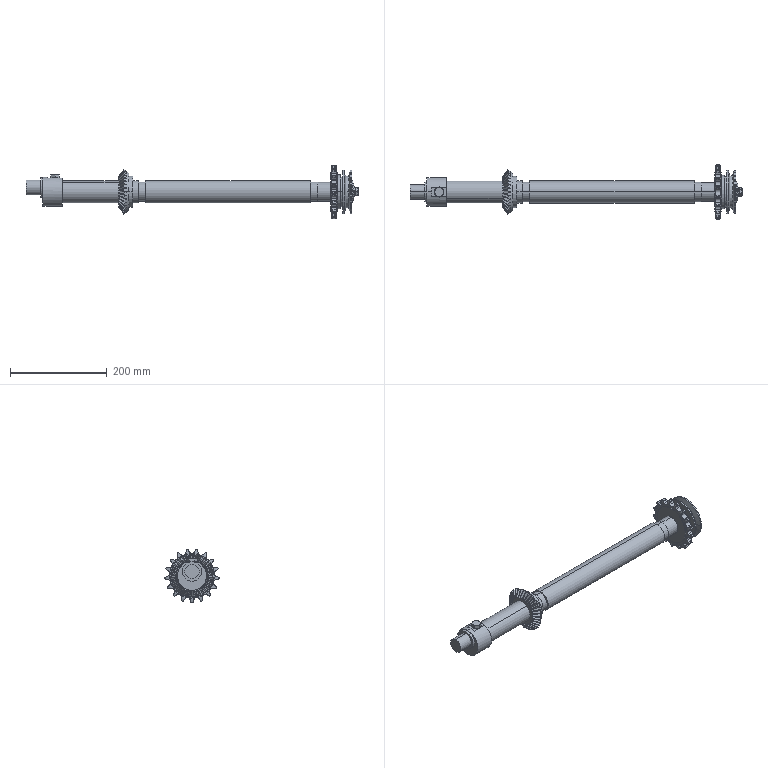Part | SolidWorks | features AEMSimFeature 1, CompositeCurve 1 | 14 solids | 782 faces | box 685.4 x 111.714 x 111.249 mm | volume 1337339 mm3 | cylinder 271 | cone 258 | plane 125 | spline 72 | torus 56 | commonest cylinder face diameters 10 x38 12 x38 17.45 x36 31.126 x35 12.07 x22 112 x17